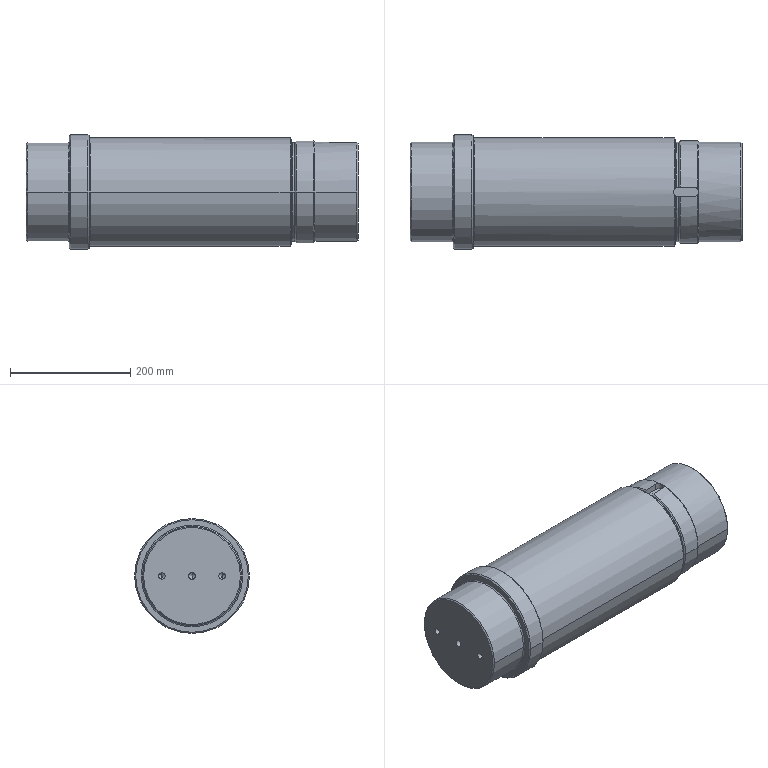Part | SolidWorks | features HoleWzd 4, Fillet 3, Chamfer 2, ICE 2, Revolution 1 | 1 solid | 79 faces | box 552 x 191 x 191 mm | volume 13392026 mm3 | cylinder 29 | cone 27 | torus 13 | plane 9 | spline 1 | commonest cylinder face diameters 165 x7 10.716 x4 16 x3 170 x3 9 x2 11.2 x2